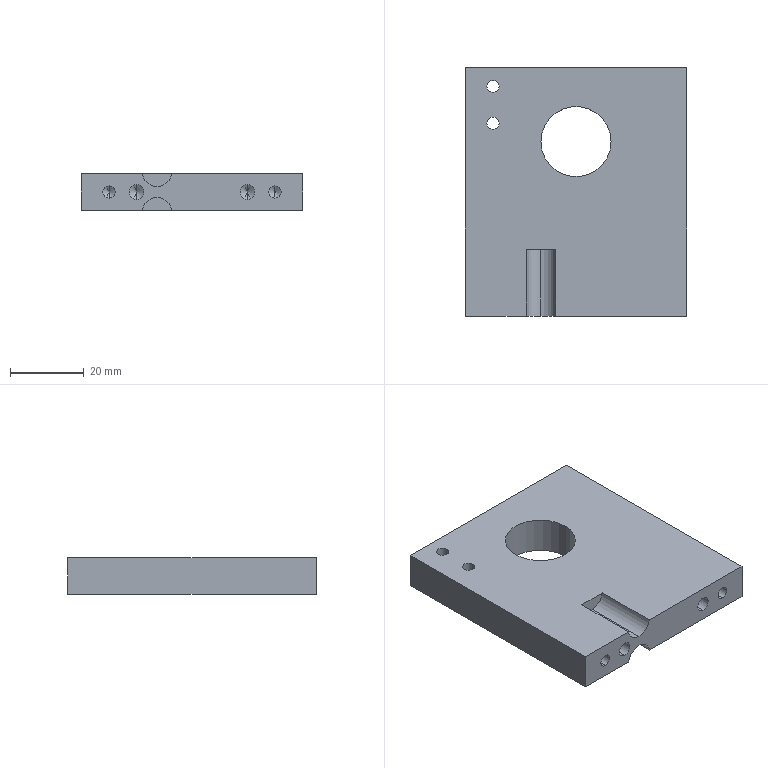Part | STEP file | 11-FG-B03511 | 1 solid | 53 faces | box 60 x 67.3 x 10 mm | volume 35980 mm3 | cylinder 27 | cone 18 | plane 8 | commonest cylinder face diameters 2.5 x10 3.3 x8 4 x4 8 x3 19 x2
STEP:
#1=CARTESIAN_POINT('',(20.5,44.7,6.5));
#2=VERTEX_POINT('',#1);
#3=CARTESIAN_POINT('',(24.469,44.7,10.));
#4=VERTEX_POINT('',#3);
#5=CARTESIAN_POINT('',(20.5,44.7,10.5));
#6=DIRECTION('',(0.,-1.,0.));
#7=DIRECTION('',(0.,0.,-1.));
#8=AXIS2_PLACEMENT_3D('',#5,#6,#7);
#9=CIRCLE('',#8,4.);
#10=EDGE_CURVE('',#2,#4,#9,.T.);
#11=ORIENTED_EDGE('',*,*,#10,.F.);
#12=CARTESIAN_POINT('',(20.5,26.7,6.5));
#13=VERTEX_POINT('',#12);
#14=CARTESIAN_POINT('',(20.5,44.7,6.5));
#15=DIRECTION('',(0.,-1.,0.));
#16=VECTOR('',#15,1000.);
#17=LINE('',#14,#16);
#18=EDGE_CURVE('',#2,#13,#17,.T.);
#19=ORIENTED_EDGE('',*,*,#18,.T.);
#20=CARTESIAN_POINT('',(24.469,26.7,10.));
#21=VERTEX_POINT('',#20);
#22=CARTESIAN_POINT('',(20.5,26.7,10.5));
#23=DIRECTION('',(0.,1.,0.));
#24=DIRECTION('',(0.,0.,1.));
#25=AXIS2_PLACEMENT_3D('',#22,#23,#24);
#26=CIRCLE('',#25,4.);
#27=EDGE_CURVE('',#21,#13,#26,.T.);
#28=ORIENTED_EDGE('',*,*,#27,.F.);
#29=CARTESIAN_POINT('',(24.469,44.7,10.));
#30=DIRECTION('',(0.,-1.,0.));
#31=VECTOR('',#30,1000.);
#32=LINE('',#29,#31);
#33=EDGE_CURVE('',#4,#21,#32,.T.);
#34=ORIENTED_EDGE('',*,*,#33,.F.);
#35=EDGE_LOOP('',(#11,#19,#28,#34));
#36=FACE_OUTER_BOUND('',#35,.T.);
#37=CARTESIAN_POINT('',(20.5,44.7,10.5));
#38=DIRECTION('',(0.,-1.,0.));
#39=DIRECTION('',(0.,0.,-1.));
#40=AXIS2_PLACEMENT_3D('',#37,#38,#39);
#41=CYLINDRICAL_SURFACE('',#40,4.);
#42=ADVANCED_FACE('',(#36),#41,.F.);
#43=CARTESIAN_POINT('',(45.,36.8,7.));
#44=VERTEX_POINT('',#43);
#45=CARTESIAN_POINT('',(45.,36.8,3.));
#46=VERTEX_POINT('',#45);
#47=CARTESIAN_POINT('',(45.,36.8,5.));
#48=DIRECTION('',(0.,-1.,0.));
#49=DIRECTION('',(0.,0.,-1.));
#50=AXIS2_PLACEMENT_3D('',#47,#48,#49);
#51=CIRCLE('',#50,2.);
#52=EDGE_CURVE('',#44,#46,#51,.T.);
#53=ORIENTED_EDGE('',*,*,#52,.F.);
#54=CARTESIAN_POINT('',(45.,26.7,7.));
#55=VERTEX_POINT('',#54);
#56=CARTESIAN_POINT('',(45.,26.7,7.));
#57=DIRECTION('',(0.,-1.,0.));
#58=VECTOR('',#57,1000.);
#59=LINE('',#56,#58);
#60=EDGE_CURVE('',#44,#55,#59,.T.);
#61=ORIENTED_EDGE('',*,*,#60,.T.);
#62=CARTESIAN_POINT('',(45.,26.7,3.));
#63=VERTEX_POINT('',#62);
#64=CARTESIAN_POINT('',(45.,26.7,5.));
#65=DIRECTION('',(0.,-1.,0.));
#66=DIRECTION('',(0.,0.,-1.));
#67=AXIS2_PLACEMENT_3D('',#64,#65,#66);
#68=CIRCLE('',#67,2.);
#69=EDGE_CURVE('',#55,#63,#68,.T.);
#70=ORIENTED_EDGE('',*,*,#69,.T.);
#71=CARTESIAN_POINT('',(45.,26.7,3.));
#72=DIRECTION('',(0.,-1.,0.));
#73=VECTOR('',#72,1000.);
#74=LINE('',#71,#73);
#75=EDGE_CURVE('',#46,#63,#74,.T.);
#76=ORIENTED_EDGE('',*,*,#75,.F.);
#77=EDGE_LOOP('',(#53,#61,#70,#76));
#78=FACE_OUTER_BOUND('',#77,.T.);
#79=CARTESIAN_POINT('',(45.,26.7,5.));
#80=DIRECTION('',(0.,-1.,0.));
#81=DIRECTION('',(0.,0.,-1.));
#82=AXIS2_PLACEMENT_3D('',#79,#80,#81);
#83=CYLINDRICAL_SURFACE('',#82,2.);
#84=ADVANCED_FACE('',(#78),#83,.F.);
#85=CARTESIAN_POINT('',(45.,38.002,5.));
#86=VERTEX_POINT('',#85);
#87=CARTESIAN_POINT('',(45.,36.8,3.));
#88=DIRECTION('',(0.,-0.515,-0.8572));
#89=VECTOR('',#88,1000.);
#90=LINE('',#87,#89);
#91=EDGE_CURVE('',#86,#46,#90,.T.);
#92=ORIENTED_EDGE('',*,*,#91,.F.);
#93=CARTESIAN_POINT('',(45.,36.8,7.));
#94=DIRECTION('',(0.,-0.515,0.8572));
#95=VECTOR('',#94,1000.);
#96=LINE('',#93,#95);
#97=EDGE_CURVE('',#86,#44,#96,.T.);
#98=ORIENTED_EDGE('',*,*,#97,.T.);
#99=ORIENTED_EDGE('',*,*,#52,.T.);
#100=EDGE_LOOP('',(#92,#98,#99));
#101=FACE_OUTER_BOUND('',#100,.T.);
#102=CARTESIAN_POINT('',(45.,36.8,5.));
#103=DIRECTION('',(0.,-1.,0.));
#104=DIRECTION('',(0.,0.,-1.));
#105=AXIS2_PLACEMENT_3D('',#102,#103,#104);
#106=CONICAL_SURFACE('',#105,2.,1.03);
#107=ADVANCED_FACE('',(#101),#106,.F.);
#108=CARTESIAN_POINT('',(15.,36.8,7.));
#109=VERTEX_POINT('',#108);
#110=CARTESIAN_POINT('',(15.,36.8,3.));
#111=VERTEX_POINT('',#110);
#112=CARTESIAN_POINT('',(15.,36.8,5.));
#113=DIRECTION('',(0.,-1.,0.));
#114=DIRECTION('',(0.,0.,-1.));
#115=AXIS2_PLACEMENT_3D('',#112,#113,#114);
#116=CIRCLE('',#115,2.);
#117=EDGE_CURVE('',#109,#111,#116,.T.);
#118=ORIENTED_EDGE('',*,*,#117,.F.);
#119=CARTESIAN_POINT('',(15.,26.7,7.));
#120=VERTEX_POINT('',#119);
#121=CARTESIAN_POINT('',(15.,26.7,7.));
#122=DIRECTION('',(0.,-1.,0.));
#123=VECTOR('',#122,1000.);
#124=LINE('',#121,#123);
#125=EDGE_CURVE('',#109,#120,#124,.T.);
#126=ORIENTED_EDGE('',*,*,#125,.T.);
#127=CARTESIAN_POINT('',(15.,26.7,3.));
#128=VERTEX_POINT('',#127);
#129=CARTESIAN_POINT('',(15.,26.7,5.));
#130=DIRECTION('',(0.,-1.,0.));
#131=DIRECTION('',(0.,0.,-1.));
#132=AXIS2_PLACEMENT_3D('',#129,#130,#131);
#133=CIRCLE('',#132,2.);
#134=EDGE_CURVE('',#120,#128,#133,.T.);
#135=ORIENTED_EDGE('',*,*,#134,.T.);
#136=CARTESIAN_POINT('',(15.,26.7,3.));
#137=DIRECTION('',(0.,-1.,0.));
#138=VECTOR('',#137,1000.);
#139=LINE('',#136,#138);
#140=EDGE_CURVE('',#111,#128,#139,.T.);
#141=ORIENTED_EDGE('',*,*,#140,.F.);
#142=EDGE_LOOP('',(#118,#126,#135,#141));
#143=FACE_OUTER_BOUND('',#142,.T.);
#144=CARTESIAN_POINT('',(15.,26.7,5.));
#145=DIRECTION('',(0.,-1.,0.));
#146=DIRECTION('',(0.,0.,-1.));
#147=AXIS2_PLACEMENT_3D('',#144,#145,#146);
#148=CYLINDRICAL_SURFACE('',#147,2.);
#149=ADVANCED_FACE('',(#143),#148,.F.);
#150=CARTESIAN_POINT('',(15.,38.002,5.));
#151=VERTEX_POINT('',#150);
#152=CARTESIAN_POINT('',(15.,36.8,3.));
#153=DIRECTION('',(0.,-0.515,-0.8572));
#154=VECTOR('',#153,1000.);
#155=LINE('',#152,#154);
#156=EDGE_CURVE('',#151,#111,#155,.T.);
#157=ORIENTED_EDGE('',*,*,#156,.F.);
#158=CARTESIAN_POINT('',(15.,36.8,7.));
#159=DIRECTION('',(0.,-0.515,0.8572));
#160=VECTOR('',#159,1000.);
#161=LINE('',#158,#160);
#162=EDGE_CURVE('',#151,#109,#161,.T.);
#163=ORIENTED_EDGE('',*,*,#162,.T.);
#164=ORIENTED_EDGE('',*,*,#117,.T.);
#165=EDGE_LOOP('',(#157,#163,#164));
#166=FACE_OUTER_BOUND('',#165,.T.);
#167=CARTESIAN_POINT('',(15.,36.8,5.));
#168=DIRECTION('',(0.,-1.,0.));
#169=DIRECTION('',(0.,0.,-1.));
#170=AXIS2_PLACEMENT_3D('',#167,#168,#169);
#171=CONICAL_SURFACE('',#170,2.,1.03);
#172=ADVANCED_FACE('',(#166),#171,.F.);
#173=CARTESIAN_POINT('',(52.5,36.8,6.65));
#174=VERTEX_POINT('',#173);
#175=CARTESIAN_POINT('',(52.5,36.8,3.35));
#176=VERTEX_POINT('',#175);
#177=CARTESIAN_POINT('',(52.5,36.8,5.));
#178=DIRECTION('',(0.,-1.,0.));
#179=DIRECTION('',(0.,0.,-1.));
#180=AXIS2_PLACEMENT_3D('',#177,#178,#179);
#181=CIRCLE('',#180,1.65);
#182=EDGE_CURVE('',#174,#176,#181,.T.);
#183=ORIENTED_EDGE('',*,*,#182,.F.);
#184=CARTESIAN_POINT('',(52.5,26.7,6.65));
#185=VERTEX_POINT('',#184);
#186=CARTESIAN_POINT('',(52.5,26.7,6.65));
#187=DIRECTION('',(0.,-1.,0.));
#188=VECTOR('',#187,1000.);
#189=LINE('',#186,#188);
#190=EDGE_CURVE('',#174,#185,#189,.T.);
#191=ORIENTED_EDGE('',*,*,#190,.T.);
#192=CARTESIAN_POINT('',(52.5,26.7,3.35));
#193=VERTEX_POINT('',#192);
#194=CARTESIAN_POINT('',(52.5,26.7,5.));
#195=DIRECTION('',(0.,-1.,0.));
#196=DIRECTION('',(0.,0.,-1.));
#197=AXIS2_PLACEMENT_3D('',#194,#195,#196);
#198=CIRCLE('',#197,1.65);
#199=EDGE_CURVE('',#185,#193,#198,.T.);
#200=ORIENTED_EDGE('',*,*,#199,.T.);
#201=CARTESIAN_POINT('',(52.5,26.7,3.35));
#202=DIRECTION('',(0.,-1.,0.));
#203=VECTOR('',#202,1000.);
#204=LINE('',#201,#203);
#205=EDGE_CURVE('',#176,#193,#204,.T.);
#206=ORIENTED_EDGE('',*,*,#205,.F.);
#207=EDGE_LOOP('',(#183,#191,#200,#206));
#208=FACE_OUTER_BOUND('',#207,.T.);
#209=CARTESIAN_POINT('',(52.5,26.7,5.));
#210=DIRECTION('',(0.,-1.,0.));
#211=DIRECTION('',(0.,0.,-1.));
#212=AXIS2_PLACEMENT_3D('',#209,#210,#211);
#213=CYLINDRICAL_SURFACE('',#212,1.65);
#214=ADVANCED_FACE('',(#208),#213,.F.);
#215=CARTESIAN_POINT('',(52.5,37.752,5.066));
#216=VERTEX_POINT('',#215);
#217=CARTESIAN_POINT('',(52.5,37.752,4.934));
#218=VERTEX_POINT('',#217);
#219=CARTESIAN_POINT('',(52.5,37.752,5.066));
#220=CARTESIAN_POINT('',(52.496,37.759,5.055));
#221=CARTESIAN_POINT('',(52.491,37.765,5.043));
#222=CARTESIAN_POINT('',(52.487,37.771,5.031));
#223=CARTESIAN_POINT('',(52.486,37.774,5.025));
#224=CARTESIAN_POINT('',(52.484,37.776,5.02));
#225=CARTESIAN_POINT('',(52.483,37.778,5.014));
#226=CARTESIAN_POINT('',(52.482,37.78,5.01));
#227=CARTESIAN_POINT('',(52.482,37.78,5.005));
#228=CARTESIAN_POINT('',(52.482,37.78,5.001));
#229=CARTESIAN_POINT('',(52.482,37.78,4.996));
#230=CARTESIAN_POINT('',(52.482,37.78,4.991));
#231=CARTESIAN_POINT('',(52.483,37.779,4.987));
#232=CARTESIAN_POINT('',(52.486,37.774,4.972));
#233=CARTESIAN_POINT('',(52.491,37.766,4.958));
#234=CARTESIAN_POINT('',(52.496,37.758,4.945));
#235=CARTESIAN_POINT('',(52.497,37.756,4.941));
#236=CARTESIAN_POINT('',(52.499,37.754,4.938));
#237=CARTESIAN_POINT('',(52.5,37.752,4.934));
#238=B_SPLINE_CURVE_WITH_KNOTS('',3,(#219,#220,#221,#222,#223,#224,#225,#226,#227,#228,#229,#230,#231,#232,#233,#234,#235,#236,#237),.UNSPECIFIED.,.F.,.F.,(4,3,3,3,3,3,4),(0.000000627,0.00004275,0.0000616,0.00007533,0.00008914,0.0001384,0.0001519),.UNSPECIFIED.);
#239=EDGE_CURVE('',#216,#218,#238,.T.);
#240=ORIENTED_EDGE('',*,*,#239,.F.);
#241=CARTESIAN_POINT('',(52.5,36.8,6.65));
#242=DIRECTION('',(0.,-0.515,0.8572));
#243=VECTOR('',#242,1000.);
#244=LINE('',#241,#243);
#245=EDGE_CURVE('',#216,#174,#244,.T.);
#246=ORIENTED_EDGE('',*,*,#245,.T.);
#247=ORIENTED_EDGE('',*,*,#182,.T.);
#248=CARTESIAN_POINT('',(52.5,36.8,3.35));
#249=DIRECTION('',(0.,-0.515,-0.8572));
#250=VECTOR('',#249,1000.);
#251=LINE('',#248,#250);
#252=EDGE_CURVE('',#218,#176,#251,.T.);
#253=ORIENTED_EDGE('',*,*,#252,.F.);
#254=EDGE_LOOP('',(#240,#246,#247,#253));
#255=FACE_OUTER_BOUND('',#254,.T.);
#256=CARTESIAN_POINT('',(52.5,36.8,5.));
#257=DIRECTION('',(0.,-1.,0.));
#258=DIRECTION('',(0.,0.,-1.));
#259=AXIS2_PLACEMENT_3D('',#256,#257,#258);
#260=CONICAL_SURFACE('',#259,1.65,1.03);
#261=ADVANCED_FACE('',(#255),#260,.F.);
#262=CARTESIAN_POINT('',(7.5,36.8,6.65));
#263=VERTEX_POINT('',#262);
#264=CARTESIAN_POINT('',(7.5,36.8,3.35));
#265=VERTEX_POINT('',#264);
#266=CARTESIAN_POINT('',(7.5,36.8,5.));
#267=DIRECTION('',(0.,-1.,0.));
#268=DIRECTION('',(0.,0.,-1.));
#269=AXIS2_PLACEMENT_3D('',#266,#267,#268);
#270=CIRCLE('',#269,1.65);
#271=EDGE_CURVE('',#263,#265,#270,.T.);
#272=ORIENTED_EDGE('',*,*,#271,.F.);
#273=CARTESIAN_POINT('',(7.5,26.7,6.65));
#274=VERTEX_POINT('',#273);
#275=CARTESIAN_POINT('',(7.5,26.7,6.65));
#276=DIRECTION('',(0.,-1.,0.));
#277=VECTOR('',#276,1000.);
#278=LINE('',#275,#277);
#279=EDGE_CURVE('',#263,#274,#278,.T.);
#280=ORIENTED_EDGE('',*,*,#279,.T.);
#281=CARTESIAN_POINT('',(7.5,26.7,3.35));
#282=VERTEX_POINT('',#281);
#283=CARTESIAN_POINT('',(7.5,26.7,5.));
#284=DIRECTION('',(0.,-1.,0.));
#285=DIRECTION('',(0.,0.,-1.));
#286=AXIS2_PLACEMENT_3D('',#283,#284,#285);
#287=CIRCLE('',#286,1.65);
#288=EDGE_CURVE('',#274,#282,#287,.T.);
#289=ORIENTED_EDGE('',*,*,#288,.T.);
#290=CARTESIAN_POINT('',(7.5,26.7,3.35));
#291=DIRECTION('',(0.,-1.,0.));
#292=VECTOR('',#291,1000.);
#293=LINE('',#290,#292);
#294=EDGE_CURVE('',#265,#282,#293,.T.);
#295=ORIENTED_EDGE('',*,*,#294,.F.);
#296=EDGE_LOOP('',(#272,#280,#289,#295));
#297=FACE_OUTER_BOUND('',#296,.T.);
#298=CARTESIAN_POINT('',(7.5,26.7,5.));
#299=DIRECTION('',(0.,-1.,0.));
#300=DIRECTION('',(0.,0.,-1.));
#301=AXIS2_PLACEMENT_3D('',#298,#299,#300);
#302=CYLINDRICAL_SURFACE('',#301,1.65);
#303=ADVANCED_FACE('',(#297),#302,.F.);
#304=CARTESIAN_POINT('',(7.5,37.791,5.));
#305=VERTEX_POINT('',#304);
#306=CARTESIAN_POINT('',(7.5,36.8,3.35));
#307=DIRECTION('',(0.,-0.515,-0.8572));
#308=VECTOR('',#307,1000.);
#309=LINE('',#306,#308);
#310=EDGE_CURVE('',#305,#265,#309,.T.);
#311=ORIENTED_EDGE('',*,*,#310,.F.);
#312=CARTESIAN_POINT('',(7.5,36.8,6.65));
#313=DIRECTION('',(0.,-0.515,0.8572));
#314=VECTOR('',#313,1000.);
#315=LINE('',#312,#314);
#316=EDGE_CURVE('',#305,#263,#315,.T.);
#317=ORIENTED_EDGE('',*,*,#316,.T.);
#318=ORIENTED_EDGE('',*,*,#271,.T.);
#319=EDGE_LOOP('',(#311,#317,#318));
#320=FACE_OUTER_BOUND('',#319,.T.);
#321=CARTESIAN_POINT('',(7.5,36.8,5.));
#322=DIRECTION('',(0.,-1.,0.));
#323=DIRECTION('',(0.,0.,-1.));
#324=AXIS2_PLACEMENT_3D('',#321,#322,#323);
#325=CONICAL_SURFACE('',#324,1.65,1.03);
#326=ADVANCED_FACE('',(#320),#325,.F.);
#327=CARTESIAN_POINT('',(52.5,39.,6.25));
#328=VERTEX_POINT('',#327);
#329=CARTESIAN_POINT('',(52.5,39.,5.));
#330=DIRECTION('',(1.,0.,0.));
#331=DIRECTION('',(0.,0.,-1.));
#332=AXIS2_PLACEMENT_3D('',#329,#330,#331);
#333=CIRCLE('',#332,1.25);
#334=EDGE_CURVE('',#328,#216,#333,.T.);
#335=ORIENTED_EDGE('',*,*,#334,.F.);
#336=CARTESIAN_POINT('',(60.,39.,6.25));
#337=VERTEX_POINT('',#336);
#338=CARTESIAN_POINT('',(60.,39.,6.25));
#339=DIRECTION('',(1.,0.,0.));
#340=VECTOR('',#339,1000.);
#341=LINE('',#338,#340);
#342=EDGE_CURVE('',#328,#337,#341,.T.);
#343=ORIENTED_EDGE('',*,*,#342,.T.);
#344=CARTESIAN_POINT('',(60.,39.,3.75));
#345=VERTEX_POINT('',#344);
#346=CARTESIAN_POINT('',(60.,39.,5.));
#347=DIRECTION('',(1.,0.,0.));
#348=DIRECTION('',(0.,0.,-1.));
#349=AXIS2_PLACEMENT_3D('',#346,#347,#348);
#350=CIRCLE('',#349,1.25);
#351=EDGE_CURVE('',#337,#345,#350,.T.);
#352=ORIENTED_EDGE('',*,*,#351,.T.);
#353=CARTESIAN_POINT('',(52.5,39.,3.75));
#354=VERTEX_POINT('',#353);
#355=CARTESIAN_POINT('',(60.,39.,3.75));
#356=DIRECTION('',(1.,0.,0.));
#357=VECTOR('',#356,1000.);
#358=LINE('',#355,#357);
#359=EDGE_CURVE('',#354,#345,#358,.T.);
#360=ORIENTED_EDGE('',*,*,#359,.F.);
#361=CARTESIAN_POINT('',(52.5,39.,5.));
#362=DIRECTION('',(1.,0.,0.));
#363=DIRECTION('',(0.,0.,-1.));
#364=AXIS2_PLACEMENT_3D('',#361,#362,#363);
#365=CIRCLE('',#364,1.25);
#366=EDGE_CURVE('',#218,#354,#365,.T.);
#367=ORIENTED_EDGE('',*,*,#366,.F.);
#368=CARTESIAN_POINT('',(52.5,37.752,4.934));
#369=CARTESIAN_POINT('',(52.505,37.752,4.934));
#370=CARTESIAN_POINT('',(52.509,37.752,4.934));
#371=CARTESIAN_POINT('',(52.514,37.752,4.935));
#372=CARTESIAN_POINT('',(52.522,37.752,4.937));
#373=CARTESIAN_POINT('',(52.529,37.751,4.94));
#374=CARTESIAN_POINT('',(52.536,37.751,4.944));
#375=CARTESIAN_POINT('',(52.543,37.751,4.948));
#376=CARTESIAN_POINT('',(52.549,37.751,4.953));
#377=CARTESIAN_POINT('',(52.554,37.751,4.959));
#378=CARTESIAN_POINT('',(52.559,37.75,4.965));
#379=CARTESIAN_POINT('',(52.563,37.75,4.972));
#380=CARTESIAN_POINT('',(52.565,37.75,4.979));
#381=CARTESIAN_POINT('',(52.568,37.75,4.986));
#382=CARTESIAN_POINT('',(52.569,37.75,4.994));
#383=CARTESIAN_POINT('',(52.569,37.75,5.001));
#384=CARTESIAN_POINT('',(52.569,37.75,5.008));
#385=CARTESIAN_POINT('',(52.567,37.75,5.015));
#386=CARTESIAN_POINT('',(52.565,37.75,5.022));
#387=CARTESIAN_POINT('',(52.563,37.75,5.029));
#388=CARTESIAN_POINT('',(52.559,37.75,5.035));
#389=CARTESIAN_POINT('',(52.554,37.751,5.04));
#390=CARTESIAN_POINT('',(52.55,37.751,5.046));
#391=CARTESIAN_POINT('',(52.544,37.751,5.051));
#392=CARTESIAN_POINT('',(52.538,37.751,5.055));
#393=CARTESIAN_POINT('',(52.532,37.751,5.059));
#394=CARTESIAN_POINT('',(52.525,37.752,5.062));
#395=CARTESIAN_POINT('',(52.517,37.752,5.064));
#396=CARTESIAN_POINT('',(52.512,37.752,5.065));
#397=CARTESIAN_POINT('',(52.506,37.752,5.066));
#398=CARTESIAN_POINT('',(52.5,37.752,5.066));
#399=B_SPLINE_CURVE_WITH_KNOTS('',3,(#368,#369,#370,#371,#372,#373,#374,#375,#376,#377,#378,#379,#380,#381,#382,#383,#384,#385,#386,#387,#388,#389,#390,#391,#392,#393,#394,#395,#396,#397,#398),.UNSPECIFIED.,.F.,.F.,(4,3,3,3,3,3,3,3,3,3,4),(0.00005605,0.00006989,0.00009398,0.0001177,0.0001407,0.0001626,0.0001839,0.0002051,0.000227,0.0002498,0.0002671),.UNSPECIFIED.);
#400=EDGE_CURVE('',#218,#216,#399,.T.);
#401=ORIENTED_EDGE('',*,*,#400,.T.);
#402=EDGE_LOOP('',(#335,#343,#352,#360,#367,#401));
#403=FACE_OUTER_BOUND('',#402,.T.);
#404=CARTESIAN_POINT('',(60.,39.,5.));
#405=DIRECTION('',(1.,0.,0.));
#406=DIRECTION('',(0.,0.,-1.));
#407=AXIS2_PLACEMENT_3D('',#404,#405,#406);
#408=CYLINDRICAL_SURFACE('',#407,1.25);
#409=ADVANCED_FACE('',(#403),#408,.F.);
#410=CARTESIAN_POINT('',(51.749,39.,5.));
#411=VERTEX_POINT('',#410);
#412=CARTESIAN_POINT('',(52.5,39.,3.75));
#413=DIRECTION('',(0.515,0.,-0.8572));
#414=VECTOR('',#413,1000.);
#415=LINE('',#412,#414);
#416=EDGE_CURVE('',#411,#354,#415,.T.);
#417=ORIENTED_EDGE('',*,*,#416,.F.);
#418=CARTESIAN_POINT('',(52.5,39.,6.25));
#419=DIRECTION('',(0.515,0.,0.8572));
#420=VECTOR('',#419,1000.);
#421=LINE('',#418,#420);
#422=EDGE_CURVE('',#411,#328,#421,.T.);
#423=ORIENTED_EDGE('',*,*,#422,.T.);
#424=ORIENTED_EDGE('',*,*,#334,.T.);
#425=ORIENTED_EDGE('',*,*,#239,.T.);
#426=ORIENTED_EDGE('',*,*,#366,.T.);
#427=EDGE_LOOP('',(#417,#423,#424,#425,#426));
#428=FACE_OUTER_BOUND('',#427,.T.);
#429=CARTESIAN_POINT('',(52.5,39.,5.));
#430=DIRECTION('',(1.,0.,0.));
#431=DIRECTION('',(0.,0.,-1.));
#432=AXIS2_PLACEMENT_3D('',#429,#430,#431);
#433=CONICAL_SURFACE('',#432,1.25,1.03);
#434=ADVANCED_FACE('',(#428),#433,.F.);
#435=CARTESIAN_POINT('',(52.5,49.,6.25));
#436=VERTEX_POINT('',#435);
#437=CARTESIAN_POINT('',(52.5,49.,3.75));
#438=VERTEX_POINT('',#437);
#439=CARTESIAN_POINT('',(52.5,49.,5.));
#440=DIRECTION('',(1.,0.,0.));
#441=DIRECTION('',(0.,0.,-1.));
#442=AXIS2_PLACEMENT_3D('',#439,#440,#441);
#443=CIRCLE('',#442,1.25);
#444=EDGE_CURVE('',#436,#438,#443,.T.);
#445=ORIENTED_EDGE('',*,*,#444,.F.);
#446=CARTESIAN_POINT('',(60.,49.,6.25));
#447=VERTEX_POINT('',#446);
#448=CARTESIAN_POINT('',(60.,49.,6.25));
#449=DIRECTION('',(1.,0.,0.));
#450=VECTOR('',#449,1000.);
#451=LINE('',#448,#450);
#452=EDGE_CURVE('',#436,#447,#451,.T.);
#453=ORIENTED_EDGE('',*,*,#452,.T.);
#454=CARTESIAN_POINT('',(60.,49.,3.75));
#455=VERTEX_POINT('',#454);
#456=CARTESIAN_POINT('',(60.,49.,5.));
#457=DIRECTION('',(1.,0.,0.));
#458=DIRECTION('',(0.,0.,-1.));
#459=AXIS2_PLACEMENT_3D('',#456,#457,#458);
#460=CIRCLE('',#459,1.25);
#461=EDGE_CURVE('',#447,#455,#460,.T.);
#462=ORIENTED_EDGE('',*,*,#461,.T.);
#463=CARTESIAN_POINT('',(60.,49.,3.75));
#464=DIRECTION('',(1.,0.,0.));
#465=VECTOR('',#464,1000.);
#466=LINE('',#463,#465);
#467=EDGE_CURVE('',#438,#455,#466,.T.);
#468=ORIENTED_EDGE('',*,*,#467,.F.);
#469=EDGE_LOOP('',(#445,#453,#462,#468));
#470=FACE_OUTER_BOUND('',#469,.T.);
#471=CARTESIAN_POINT('',(60.,49.,5.));
#472=DIRECTION('',(1.,0.,0.));
#473=DIRECTION('',(0.,0.,-1.));
#474=AXIS2_PLACEMENT_3D('',#471,#472,#473);
#475=CYLINDRICAL_SURFACE('',#474,1.25);
#476=ADVANCED_FACE('',(#470),#475,.F.);
#477=CARTESIAN_POINT('',(51.749,49.,5.));
#478=VERTEX_POINT('',#477);
#479=CARTESIAN_POINT('',(52.5,49.,3.75));
#480=DIRECTION('',(0.515,0.,-0.8572));
#481=VECTOR('',#480,1000.);
#482=LINE('',#479,#481);
#483=EDGE_CURVE('',#478,#438,#482,.T.);
#484=ORIENTED_EDGE('',*,*,#483,.F.);
#485=CARTESIAN_POINT('',(52.5,49.,6.25));
#486=DIRECTION('',(0.515,0.,0.8572));
#487=VECTOR('',#486,1000.);
#488=LINE('',#485,#487);
#489=EDGE_CURVE('',#478,#436,#488,.T.);
#490=ORIENTED_EDGE('',*,*,#489,.T.);
#491=ORIENTED_EDGE('',*,*,#444,.T.);
#492=EDGE_LOOP('',(#484,#490,#491));
#493=FACE_OUTER_BOUND('',#492,.T.);
#494=CARTESIAN_POINT('',(52.5,49.,5.));
#495=DIRECTION('',(1.,0.,0.));
#496=DIRECTION('',(0.,0.,-1.));
#497=AXIS2_PLACEMENT_3D('',#494,#495,#496);
#498=CONICAL_SURFACE('',#497,1.25,1.03);
#499=ADVANCED_FACE('',(#493),#498,.F.);
#500=CARTESIAN_POINT('',(52.5,59.,6.25));
#501=VERTEX_POINT('',#500);
#502=CARTESIAN_POINT('',(52.5,59.,3.75));
#503=VERTEX_POINT('',#502);
#504=CARTESIAN_POINT('',(52.5,59.,5.));
#505=DIRECTION('',(1.,0.,0.));
#506=DIRECTION('',(0.,0.,-1.));
#507=AXIS2_PLACEMENT_3D('',#504,#505,#506);
#508=CIRCLE('',#507,1.25);
#509=EDGE_CURVE('',#501,#503,#508,.T.);
#510=ORIENTED_EDGE('',*,*,#509,.F.);
#511=CARTESIAN_POINT('',(60.,59.,6.25));
#512=VERTEX_POINT('',#511);
#513=CARTESIAN_POINT('',(60.,59.,6.25));
#514=DIRECTION('',(1.,0.,0.));
#515=VECTOR('',#514,1000.);
#516=LINE('',#513,#515);
#517=EDGE_CURVE('',#501,#512,#516,.T.);
#518=ORIENTED_EDGE('',*,*,#517,.T.);
#519=CARTESIAN_POINT('',(60.,59.,3.75));
#520=VERTEX_POINT('',#519);
#521=CARTESIAN_POINT('',(60.,59.,5.));
#522=DIRECTION('',(1.,0.,0.));
#523=DIRECTION('',(0.,0.,-1.));
#524=AXIS2_PLACEMENT_3D('',#521,#522,#523);
#525=CIRCLE('',#524,1.25);
#526=EDGE_CURVE('',#512,#520,#525,.T.);
#527=ORIENTED_EDGE('',*,*,#526,.T.);
#528=CARTESIAN_POINT('',(60.,59.,3.75));
#529=DIRECTION('',(1.,0.,0.));
#530=VECTOR('',#529,1000.);
#531=LINE('',#528,#530);
#532=EDGE_CURVE('',#503,#520,#531,.T.);
#533=ORIENTED_EDGE('',*,*,#532,.F.);
#534=EDGE_LOOP('',(#510,#518,#527,#533));
#535=FACE_OUTER_BOUND('',#534,.T.);
#536=CARTESIAN_POINT('',(60.,59.,5.));
#537=DIRECTION('',(1.,0.,0.));
#538=DIRECTION('',(0.,0.,-1.));
#539=AXIS2_PLACEMENT_3D('',#536,#537,#538);
#540=CYLINDRICAL_SURFACE('',#539,1.25);
#541=ADVANCED_FACE('',(#535),#540,.F.);
#542=CARTESIAN_POINT('',(51.749,59.,5.));
#543=VERTEX_POINT('',#542);
#544=CARTESIAN_POINT('',(52.5,59.,3.75));
#545=DIRECTION('',(0.515,0.,-0.8572));
#546=VECTOR('',#545,1000.);
#547=LINE('',#544,#546);
#548=EDGE_CURVE('',#543,#503,#547,.T.);
#549=ORIENTED_EDGE('',*,*,#548,.F.);
#550=CARTESIAN_POINT('',(52.5,59.,6.25));
#551=DIRECTION('',(0.515,0.,0.8572));
#552=VECTOR('',#551,1000.);
#553=LINE('',#550,#552);
#554=EDGE_CURVE('',#543,#501,#553,.T.);
#555=ORIENTED_EDGE('',*,*,#554,.T.);
#556=ORIENTED_EDGE('',*,*,#509,.T.);
#557=EDGE_LOOP('',(#549,#555,#556));
#558=FACE_OUTER_BOUND('',#557,.T.);
#559=CARTESIAN_POINT('',(52.5,59.,5.));
#560=DIRECTION('',(1.,0.,0.));
#561=DIRECTION('',(0.,0.,-1.));
#562=AXIS2_PLACEMENT_3D('',#559,#560,#561);
#563=CONICAL_SURFACE('',#562,1.25,1.03);
#564=ADVANCED_FACE('',(#558),#563,.F.);
#565=CARTESIAN_POINT('',(52.5,69.,6.25));
#566=VERTEX_POINT('',#565);
#567=CARTESIAN_POINT('',(52.5,69.,3.75));
#568=VERTEX_POINT('',#567);
#569=CARTESIAN_POINT('',(52.5,69.,5.));
#570=DIRECTION('',(1.,0.,0.));
#571=DIRECTION('',(0.,0.,-1.));
#572=AXIS2_PLACEMENT_3D('',#569,#570,#571);
#573=CIRCLE('',#572,1.25);
#574=EDGE_CURVE('',#566,#568,#573,.T.);
#575=ORIENTED_EDGE('',*,*,#574,.F.);
#576=CARTESIAN_POINT('',(60.,69.,6.25));
#577=VERTEX_POINT('',#576);
#578=CARTESIAN_POINT('',(60.,69.,6.25));
#579=DIRECTION('',(1.,0.,0.));
#580=VECTOR('',#579,1000.);
#581=LINE('',#578,#580);
#582=EDGE_CURVE('',#566,#577,#581,.T.);
#583=ORIENTED_EDGE('',*,*,#582,.T.);
#584=CARTESIAN_POINT('',(60.,69.,3.75));
#585=VERTEX_POINT('',#584);
#586=CARTESIAN_POINT('',(60.,69.,5.));
#587=DIRECTION('',(1.,0.,0.));
#588=DIRECTION('',(0.,0.,-1.));
#589=AXIS2_PLACEMENT_3D('',#586,#587,#588);
#590=CIRCLE('',#589,1.25);
#591=EDGE_CURVE('',#577,#585,#590,.T.);
#592=ORIENTED_EDGE('',*,*,#591,.T.);
#593=CARTESIAN_POINT('',(60.,69.,3.75));
#594=DIRECTION('',(1.,0.,0.));
#595=VECTOR('',#594,1000.);
#596=LINE('',#593,#595);
#597=EDGE_CURVE('',#568,#585,#596,.T.);
#598=ORIENTED_EDGE('',*,*,#597,.F.);
#599=EDGE_LOOP('',(#575,#583,#592,#598));
#600=FACE_OUTER_BOUND('',#599,.T.);
#601=CARTESIAN_POINT('',(60.,69.,5.));
#602=DIRECTION('',(1.,0.,0.));
#603=DIRECTION('',(0.,0.,-1.));
#604=AXIS2_PLACEMENT_3D('',#601,#602,#603);
#605=CYLINDRICAL_SURFACE('',#604,1.25);
#606=ADVANCED_FACE('',(#600),#605,.F.);
#607=CARTESIAN_POINT('',(51.749,69.,5.));
#608=VERTEX_POINT('',#607);
#609=CARTESIAN_POINT('',(52.5,69.,3.75));
#610=DIRECTION('',(0.515,0.,-0.8572));
#611=VECTOR('',#610,1000.);
#612=LINE('',#609,#611);
#613=EDGE_CURVE('',#608,#568,#612,.T.);
#614=ORIENTED_EDGE('',*,*,#613,.F.);
#615=CARTESIAN_POINT('',(52.5,69.,6.25));
#616=DIRECTION('',(0.515,0.,0.8572));
#617=VECTOR('',#616,1000.);
#618=LINE('',#615,#617);
#619=EDGE_CURVE('',#608,#566,#618,.T.);
#620=ORIENTED_EDGE('',*,*,#619,.T.);
#621=ORIENTED_EDGE('',*,*,#574,.T.);
#622=EDGE_LOOP('',(#614,#620,#621));
#623=FACE_OUTER_BOUND('',#622,.T.);
#624=CARTESIAN_POINT('',(52.5,69.,5.));
#625=DIRECTION('',(1.,0.,0.));
#626=DIRECTION('',(0.,0.,-1.));
#627=AXIS2_PLACEMENT_3D('',#624,#625,#626);
#628=CONICAL_SURFACE('',#627,1.25,1.03);
#629=ADVANCED_FACE('',(#623),#628,.F.);
#630=CARTESIAN_POINT('',(52.5,79.,6.25));
#631=VERTEX_POINT('',#630);
#632=CARTESIAN_POINT('',(52.5,79.,3.75));
#633=VERTEX_POINT('',#632);
#634=CARTESIAN_POINT('',(52.5,79.,5.));
#635=DIRECTION('',(1.,0.,0.));
#636=DIRECTION('',(0.,0.,-1.));
#637=AXIS2_PLACEMENT_3D('',#634,#635,#636);
#638=CIRCLE('',#637,1.25);
#639=EDGE_CURVE('',#631,#633,#638,.T.);
#640=ORIENTED_EDGE('',*,*,#639,.F.);
#641=CARTESIAN_POINT('',(60.,79.,6.25));
#642=VERTEX_POINT('',#641);
#643=CARTESIAN_POINT('',(60.,79.,6.25));
#644=DIRECTION('',(1.,0.,0.));
#645=VECTOR('',#644,1000.);
#646=LINE('',#643,#645);
#647=EDGE_CURVE('',#631,#642,#646,.T.);
#648=ORIENTED_EDGE('',*,*,#647,.T.);
#649=CARTESIAN_POINT('',(60.,79.,3.75));
#650=VERTEX_POINT('',#649);
#651=CARTESIAN_POINT('',(60.,79.,5.));
#652=DIRECTION('',(1.,0.,0.));
#653=DIRECTION('',(0.,0.,-1.));
#654=AXIS2_PLACEMENT_3D('',#651,#652,#653);
#655=CIRCLE('',#654,1.25);
#656=EDGE_CURVE('',#642,#650,#655,.T.);
#657=ORIENTED_EDGE('',*,*,#656,.T.);
#658=CARTESIAN_POINT('',(60.,79.,3.75));
#659=DIRECTION('',(1.,0.,0.));
#660=VECTOR('',#659,1000.);
#661=LINE('',#658,#660);
#662=EDGE_CURVE('',#633,#650,#661,.T.);
#663=ORIENTED_EDGE('',*,*,#662,.F.);
#664=EDGE_LOOP('',(#640,#648,#657,#663));
#665=FACE_OUTER_BOUND('',#664,.T.);
#666=CARTESIAN_POINT('',(60.,79.,5.));
#667=DIRECTION('',(1.,0.,0.));
#668=DIRECTION('',(0.,0.,-1.));
#669=AXIS2_PLACEMENT_3D('',#666,#667,#668);
#670=CYLINDRICAL_SURFACE('',#669,1.25);
#671=ADVANCED_FACE('',(#665),#670,.F.);
#672=CARTESIAN_POINT('',(51.749,79.,5.));
#673=VERTEX_POINT('',#672);
#674=CARTESIAN_POINT('',(52.5,79.,3.75));
#675=DIRECTION('',(0.515,0.,-0.8572));
#676=VECTOR('',#675,1000.);
#677=LINE('',#674,#676);
#678=EDGE_CURVE('',#673,#633,#677,.T.);
#679=ORIENTED_EDGE('',*,*,#678,.F.);
#680=CARTESIAN_POINT('',(52.5,79.,6.25));
#681=DIRECTION('',(0.515,0.,0.8572));
#682=VECTOR('',#681,1000.);
#683=LINE('',#680,#682);
#684=EDGE_CURVE('',#673,#631,#683,.T.);
#685=ORIENTED_EDGE('',*,*,#684,.T.);
#686=ORIENTED_EDGE('',*,*,#639,.T.);
#687=EDGE_LOOP('',(#679,#685,#686));
#688=FACE_OUTER_BOUND('',#687,.T.);
#689=CARTESIAN_POINT('',(52.5,79.,5.));
#690=DIRECTION('',(1.,0.,0.));
#691=DIRECTION('',(0.,0.,-1.));
#692=AXIS2_PLACEMENT_3D('',#689,#690,#691);
#693=CONICAL_SURFACE('',#692,1.25,1.03);
#694=ADVANCED_FACE('',(#688),#693,.F.);
#695=CARTESIAN_POINT('',(9.15,89.,10.));
#696=VERTEX_POINT('',#695);
#697=CARTESIAN_POINT('',(5.85,89.,10.));
#698=VERTEX_POINT('',#697);
#699=CARTESIAN_POINT('',(7.5,89.,10.));
#700=DIRECTION('',(0.,0.,-1.));
#701=DIRECTION('',(-1.,0.,0.));
#702=AXIS2_PLACEMENT_3D('',#699,#700,#701);
#703=CIRCLE('',#702,1.65);
#704=EDGE_CURVE('',#696,#698,#703,.T.);
#705=ORIENTED_EDGE('',*,*,#704,.F.);
#706=CARTESIAN_POINT('',(9.15,89.,0.));
#707=VERTEX_POINT('',#706);
#708=CARTESIAN_POINT('',(9.15,89.,0.));
#709=DIRECTION('',(0.,0.,-1.));
#710=VECTOR('',#709,1000.);
#711=LINE('',#708,#710);
#712=EDGE_CURVE('',#696,#707,#711,.T.);
#713=ORIENTED_EDGE('',*,*,#712,.T.);
#714=CARTESIAN_POINT('',(5.85,89.,0.));
#715=VERTEX_POINT('',#714);
#716=CARTESIAN_POINT('',(7.5,89.,0.));
#717=DIRECTION('',(0.,0.,-1.));
#718=DIRECTION('',(-1.,0.,0.));
#719=AXIS2_PLACEMENT_3D('',#716,#717,#718);
#720=CIRCLE('',#719,1.65);
#721=EDGE_CURVE('',#707,#715,#720,.T.);
#722=ORIENTED_EDGE('',*,*,#721,.T.);
#723=CARTESIAN_POINT('',(5.85,89.,0.));
#724=DIRECTION('',(0.,0.,-1.));
#725=VECTOR('',#724,1000.);
#726=LINE('',#723,#725);
#727=EDGE_CURVE('',#698,#715,#726,.T.);
#728=ORIENTED_EDGE('',*,*,#727,.F.);
#729=EDGE_LOOP('',(#705,#713,#722,#728));
#730=FACE_OUTER_BOUND('',#729,.T.);
#731=CARTESIAN_POINT('',(7.5,89.,0.));
#732=DIRECTION('',(0.,0.,-1.));
#733=DIRECTION('',(-1.,0.,0.));
#734=AXIS2_PLACEMENT_3D('',#731,#732,#733);
#735=CYLINDRICAL_SURFACE('',#734,1.65);
#736=ADVANCED_FACE('',(#730),#735,.F.);
#737=CARTESIAN_POINT('',(9.15,79.,10.));
#738=VERTEX_POINT('',#737);
#739=CARTESIAN_POINT('',(5.85,79.,10.));
#740=VERTEX_POINT('',#739);
#741=CARTESIAN_POINT('',(7.5,79.,10.));
#742=DIRECTION('',(0.,0.,-1.));
#743=DIRECTION('',(-1.,0.,0.));
#744=AXIS2_PLACEMENT_3D('',#741,#742,#743);
#745=CIRCLE('',#744,1.65);
#746=EDGE_CURVE('',#738,#740,#745,.T.);
#747=ORIENTED_EDGE('',*,*,#746,.F.);
#748=CARTESIAN_POINT('',(9.15,79.,0.));
#749=VERTEX_POINT('',#748);
#750=CARTESIAN_POINT('',(9.15,79.,0.));
#751=DIRECTION('',(0.,0.,-1.));
#752=VECTOR('',#751,1000.);
#753=LINE('',#750,#752);
#754=EDGE_CURVE('',#738,#749,#753,.T.);
#755=ORIENTED_EDGE('',*,*,#754,.T.);
#756=CARTESIAN_POINT('',(5.85,79.,0.));
#757=VERTEX_POINT('',#756);
#758=CARTESIAN_POINT('',(7.5,79.,0.));
#759=DIRECTION('',(0.,0.,-1.));
#760=DIRECTION('',(-1.,0.,0.));
#761=AXIS2_PLACEMENT_3D('',#758,#759,#760);
#762=CIRCLE('',#761,1.65);
#763=EDGE_CURVE('',#749,#757,#762,.T.);
#764=ORIENTED_EDGE('',*,*,#763,.T.);
#765=CARTESIAN_POINT('',(5.85,79.,0.));
#766=DIRECTION('',(0.,0.,-1.));
#767=VECTOR('',#766,1000.);
#768=LINE('',#765,#767);
#769=EDGE_CURVE('',#740,#757,#768,.T.);
#770=ORIENTED_EDGE('',*,*,#769,.F.);
#771=EDGE_LOOP('',(#747,#755,#764,#770));
#772=FACE_OUTER_BOUND('',#771,.T.);
#773=CARTESIAN_POINT('',(7.5,79.,0.));
#774=DIRECTION('',(0.,0.,-1.));
#775=DIRECTION('',(-1.,0.,0.));
#776=AXIS2_PLACEMENT_3D('',#773,#774,#775);
#777=CYLINDRICAL_SURFACE('',#776,1.65);
#778=ADVANCED_FACE('',(#772),#777,.F.);
#779=CARTESIAN_POINT('',(20.5,74.,10.));
#780=VERTEX_POINT('',#779);
#781=CARTESIAN_POINT('',(39.5,74.,10.));
#782=VERTEX_POINT('',#781);
#783=CARTESIAN_POINT('',(30.,74.,10.));
#784=DIRECTION('',(0.,0.,1.));
#785=DIRECTION('',(1.,0.,0.));
#786=AXIS2_PLACEMENT_3D('',#783,#784,#785);
#787=CIRCLE('',#786,9.5);
#788=EDGE_CURVE('',#780,#782,#787,.T.);
#789=ORIENTED_EDGE('',*,*,#788,.T.);
#790=CARTESIAN_POINT('',(39.5,74.,0.));
#791=VERTEX_POINT('',#790);
#792=CARTESIAN_POINT('',(39.5,74.,10.));
#793=DIRECTION('',(0.,0.,-1.));
#794=VECTOR('',#793,1000.);
#795=LINE('',#792,#794);
#796=EDGE_CURVE('',#782,#791,#795,.T.);
#797=ORIENTED_EDGE('',*,*,#796,.T.);
#798=CARTESIAN_POINT('',(20.5,74.,0.));
#799=VERTEX_POINT('',#798);
#800=CARTESIAN_POINT('',(30.,74.,0.));
#801=DIRECTION('',(0.,0.,1.));
#802=DIRECTION('',(1.,0.,0.));
#803=AXIS2_PLACEMENT_3D('',#800,#801,#802);
#804=CIRCLE('',#803,9.5);
#805=EDGE_CURVE('',#799,#791,#804,.T.);
#806=ORIENTED_EDGE('',*,*,#805,.F.);
#807=CARTESIAN_POINT('',(20.5,74.,10.));
#808=DIRECTION('',(0.,0.,-1.));
#809=VECTOR('',#808,1000.);
#810=LINE('',#807,#809);
#811=EDGE_CURVE('',#780,#799,#810,.T.);
#812=ORIENTED_EDGE('',*,*,#811,.F.);
#813=EDGE_LOOP('',(#789,#797,#806,#812));
#814=FACE_OUTER_BOUND('',#813,.T.);
#815=CARTESIAN_POINT('',(30.,74.,10.));
#816=DIRECTION('',(0.,0.,-1.));
#817=DIRECTION('',(-1.,0.,0.));
#818=AXIS2_PLACEMENT_3D('',#815,#816,#817);
#819=CYLINDRICAL_SURFACE('',#818,9.5);
#820=ADVANCED_FACE('',(#814),#819,.F.);
#821=CARTESIAN_POINT('',(7.5,89.,10.));
#822=DIRECTION('',(0.,0.,-1.));
#823=DIRECTION('',(-1.,0.,0.));
#824=AXIS2_PLACEMENT_3D('',#821,#822,#823);
#825=CIRCLE('',#824,1.65);
#826=EDGE_CURVE('',#698,#696,#825,.T.);
#827=ORIENTED_EDGE('',*,*,#826,.T.);
#828=ORIENTED_EDGE('',*,*,#704,.T.);
#829=EDGE_LOOP('',(#827,#828));
#830=FACE_BOUND('',#829,.T.);
#831=CARTESIAN_POINT('',(7.5,79.,10.));
#832=DIRECTION('',(0.,0.,-1.));
#833=DIRECTION('',(-1.,0.,0.));
#834=AXIS2_PLACEMENT_3D('',#831,#832,#833);
#835=CIRCLE('',#834,1.65);
#836=EDGE_CURVE('',#740,#738,#835,.T.);
#837=ORIENTED_EDGE('',*,*,#836,.T.);
#838=ORIENTED_EDGE('',*,*,#746,.T.);
#839=EDGE_LOOP('',(#837,#838));
#840=FACE_BOUND('',#839,.T.);
#841=CARTESIAN_POINT('',(16.531,44.7,10.));
#842=VERTEX_POINT('',#841);
#843=CARTESIAN_POINT('',(0.,44.7,10.));
#844=DIRECTION('',(-1.,0.,0.));
#845=VECTOR('',#844,1000.);
#846=LINE('',#843,#845);
#847=EDGE_CURVE('',#4,#842,#846,.T.);
#848=ORIENTED_EDGE('',*,*,#847,.F.);
#849=ORIENTED_EDGE('',*,*,#33,.T.);
#850=CARTESIAN_POINT('',(60.,26.7,10.));
#851=VERTEX_POINT('',#850);
#852=CARTESIAN_POINT('',(0.,26.7,10.));
#853=DIRECTION('',(1.,0.,0.));
#854=VECTOR('',#853,1000.);
#855=LINE('',#852,#854);
#856=EDGE_CURVE('',#21,#851,#855,.T.);
#857=ORIENTED_EDGE('',*,*,#856,.T.);
#858=CARTESIAN_POINT('',(60.,94.,10.));
#859=VERTEX_POINT('',#858);
#860=CARTESIAN_POINT('',(60.,0.,10.));
#861=DIRECTION('',(0.,1.,0.));
#862=VECTOR('',#861,1000.);
#863=LINE('',#860,#862);
#864=EDGE_CURVE('',#851,#859,#863,.T.);
#865=ORIENTED_EDGE('',*,*,#864,.T.);
#866=CARTESIAN_POINT('',(0.,94.,10.));
#867=VERTEX_POINT('',#866);
#868=CARTESIAN_POINT('',(0.,94.,10.));
#869=DIRECTION('',(-1.,0.,0.));
#870=VECTOR('',#869,1000.);
#871=LINE('',#868,#870);
#872=EDGE_CURVE('',#859,#867,#871,.T.);
#873=ORIENTED_EDGE('',*,*,#872,.T.);
#874=CARTESIAN_POINT('',(0.,26.7,10.));
#875=VERTEX_POINT('',#874);
#876=CARTESIAN_POINT('',(0.,0.,10.));
#877=DIRECTION('',(0.,-1.,0.));
#878=VECTOR('',#877,1000.);
#879=LINE('',#876,#878);
#880=EDGE_CURVE('',#867,#875,#879,.T.);
#881=ORIENTED_EDGE('',*,*,#880,.T.);
#882=CARTESIAN_POINT('',(16.531,26.7,10.));
#883=VERTEX_POINT('',#882);
#884=CARTESIAN_POINT('',(0.,26.7,10.));
#885=DIRECTION('',(1.,0.,0.));
#886=VECTOR('',#885,1000.);
#887=LINE('',#884,#886);
#888=EDGE_CURVE('',#875,#883,#887,.T.);
#889=ORIENTED_EDGE('',*,*,#888,.T.);
#890=CARTESIAN_POINT('',(16.531,44.7,10.));
#891=DIRECTION('',(0.,1.,0.));
#892=VECTOR('',#891,1000.);
#893=LINE('',#890,#892);
#894=EDGE_CURVE('',#883,#842,#893,.T.);
#895=ORIENTED_EDGE('',*,*,#894,.T.);
#896=EDGE_LOOP('',(#848,#849,#857,#865,#873,#881,#889,#895));
#897=FACE_OUTER_BOUND('',#896,.T.);
#898=ORIENTED_EDGE('',*,*,#788,.F.);
#899=CARTESIAN_POINT('',(30.,74.,10.));
#900=DIRECTION('',(0.,0.,1.));
#901=DIRECTION('',(1.,0.,0.));
#902=AXIS2_PLACEMENT_3D('',#899,#900,#901);
#903=CIRCLE('',#902,9.5);
#904=EDGE_CURVE('',#782,#780,#903,.T.);
#905=ORIENTED_EDGE('',*,*,#904,.F.);
#906=EDGE_LOOP('',(#898,#905));
#907=FACE_BOUND('',#906,.T.);
#908=CARTESIAN_POINT('',(0.,94.,10.));
#909=DIRECTION('',(0.,0.,-1.));
#910=DIRECTION('',(-1.,0.,0.));
#911=AXIS2_PLACEMENT_3D('',#908,#909,#910);
#912=PLANE('',#911);
#913=ADVANCED_FACE('',(#830,#840,#897,#907),#912,.F.);
#914=CARTESIAN_POINT('',(24.469,44.7,0.));
#915=VERTEX_POINT('',#914);
#916=CARTESIAN_POINT('',(24.469,26.7,0.));
#917=VERTEX_POINT('',#916);
#918=CARTESIAN_POINT('',(24.469,44.7,0.));
#919=DIRECTION('',(0.,-1.,0.));
#920=VECTOR('',#919,1000.);
#921=LINE('',#918,#920);
#922=EDGE_CURVE('',#915,#917,#921,.T.);
#923=ORIENTED_EDGE('',*,*,#922,.F.);
#924=CARTESIAN_POINT('',(16.531,44.7,0.));
#925=VERTEX_POINT('',#924);
#926=CARTESIAN_POINT('',(0.,44.7,0.));
#927=DIRECTION('',(1.,0.,0.));
#928=VECTOR('',#927,1000.);
#929=LINE('',#926,#928);
#930=EDGE_CURVE('',#925,#915,#929,.T.);
#931=ORIENTED_EDGE('',*,*,#930,.F.);
#932=CARTESIAN_POINT('',(16.531,26.7,0.));
#933=VERTEX_POINT('',#932);
#934=CARTESIAN_POINT('',(16.531,44.7,0.));
#935=DIRECTION('',(0.,1.,0.));
#936=VECTOR('',#935,1000.);
#937=LINE('',#934,#936);
#938=EDGE_CURVE('',#933,#925,#937,.T.);
#939=ORIENTED_EDGE('',*,*,#938,.F.);
#940=CARTESIAN_POINT('',(0.,26.7,0.));
#941=VERTEX_POINT('',#940);
#942=CARTESIAN_POINT('',(72.,26.7,0.));
#943=DIRECTION('',(1.,0.,0.));
#944=VECTOR('',#943,1000.);
#945=LINE('',#942,#944);
#946=EDGE_CURVE('',#941,#933,#945,.T.);
#947=ORIENTED_EDGE('',*,*,#946,.F.);
#948=CARTESIAN_POINT('',(0.,94.,0.));
#949=VERTEX_POINT('',#948);
#950=CARTESIAN_POINT('',(0.,0.,0.));
#951=DIRECTION('',(0.,-1.,0.));
#952=VECTOR('',#951,1000.);
#953=LINE('',#950,#952);
#954=EDGE_CURVE('',#949,#941,#953,.T.);
#955=ORIENTED_EDGE('',*,*,#954,.F.);
#956=CARTESIAN_POINT('',(60.,94.,0.));
#957=VERTEX_POINT('',#956);
#958=CARTESIAN_POINT('',(0.,94.,0.));
#959=DIRECTION('',(-1.,0.,0.));
#960=VECTOR('',#959,1000.);
#961=LINE('',#958,#960);
#962=EDGE_CURVE('',#957,#949,#961,.T.);
#963=ORIENTED_EDGE('',*,*,#962,.F.);
#964=CARTESIAN_POINT('',(60.,26.7,0.));
#965=VERTEX_POINT('',#964);
#966=CARTESIAN_POINT('',(60.,0.,0.));
#967=DIRECTION('',(0.,1.,0.));
#968=VECTOR('',#967,1000.);
#969=LINE('',#966,#968);
#970=EDGE_CURVE('',#965,#957,#969,.T.);
#971=ORIENTED_EDGE('',*,*,#970,.F.);
#972=CARTESIAN_POINT('',(72.,26.7,0.));
#973=DIRECTION('',(1.,0.,0.));
#974=VECTOR('',#973,1000.);
#975=LINE('',#972,#974);
#976=EDGE_CURVE('',#917,#965,#975,.T.);
#977=ORIENTED_EDGE('',*,*,#976,.F.);
#978=EDGE_LOOP('',(#923,#931,#939,#947,#955,#963,#971,#977));
#979=FACE_OUTER_BOUND('',#978,.T.);
#980=CARTESIAN_POINT('',(7.5,89.,0.));
#981=DIRECTION('',(0.,0.,-1.));
#982=DIRECTION('',(-1.,0.,0.));
#983=AXIS2_PLACEMENT_3D('',#980,#981,#982);
#984=CIRCLE('',#983,1.65);
#985=EDGE_CURVE('',#715,#707,#984,.T.);
#986=ORIENTED_EDGE('',*,*,#985,.F.);
#987=ORIENTED_EDGE('',*,*,#721,.F.);
#988=EDGE_LOOP('',(#986,#987));
#989=FACE_BOUND('',#988,.T.);
#990=CARTESIAN_POINT('',(7.5,79.,0.));
#991=DIRECTION('',(0.,0.,-1.));
#992=DIRECTION('',(-1.,0.,0.));
#993=AXIS2_PLACEMENT_3D('',#990,#991,#992);
#994=CIRCLE('',#993,1.65);
#995=EDGE_CURVE('',#757,#749,#994,.T.);
#996=ORIENTED_EDGE('',*,*,#995,.F.);
#997=ORIENTED_EDGE('',*,*,#763,.F.);
#998=EDGE_LOOP('',(#996,#997));
#999=FACE_BOUND('',#998,.T.);
#1000=ORIENTED_EDGE('',*,*,#805,.T.);
#1001=CARTESIAN_POINT('',(30.,74.,0.));
#1002=DIRECTION('',(0.,0.,1.));
#1003=DIRECTION('',(1.,0.,0.));
#1004=AXIS2_PLACEMENT_3D('',#1001,#1002,#1003);
#1005=CIRCLE('',#1004,9.5);
#1006=EDGE_CURVE('',#791,#799,#1005,.T.);
#1007=ORIENTED_EDGE('',*,*,#1006,.T.);
#1008=EDGE_LOOP('',(#1000,#1007));
#1009=FACE_BOUND('',#1008,.T.);
#1010=CARTESIAN_POINT('',(0.,94.,0.));
#1011=DIRECTION('',(0.,0.,-1.));
#1012=DIRECTION('',(-1.,0.,0.));
#1013=AXIS2_PLACEMENT_3D('',#1010,#1011,#1012);
#1014=PLANE('',#1013);
#1015=ADVANCED_FACE('',(#979,#989,#999,#1009),#1014,.T.);
#1016=ORIENTED_EDGE('',*,*,#954,.T.);
#1017=CARTESIAN_POINT('',(0.,26.7,10.));
#1018=DIRECTION('',(0.,0.,-1.));
#1019=VECTOR('',#1018,1000.);
#1020=LINE('',#1017,#1019);
#1021=EDGE_CURVE('',#875,#941,#1020,.T.);
#1022=ORIENTED_EDGE('',*,*,#1021,.F.);
#1023=ORIENTED_EDGE('',*,*,#880,.F.);
#1024=CARTESIAN_POINT('',(0.,94.,10.));
#1025=DIRECTION('',(0.,0.,-1.));
#1026=VECTOR('',#1025,1000.);
#1027=LINE('',#1024,#1026);
#1028=EDGE_CURVE('',#867,#949,#1027,.T.);
#1029=ORIENTED_EDGE('',*,*,#1028,.T.);
#1030=EDGE_LOOP('',(#1016,#1022,#1023,#1029));
#1031=FACE_OUTER_BOUND('',#1030,.T.);
#1032=CARTESIAN_POINT('',(0.,0.,10.));
#1033=DIRECTION('',(1.,0.,0.));
#1034=DIRECTION('',(0.,1.,0.));
#1035=AXIS2_PLACEMENT_3D('',#1032,#1033,#1034);
#1036=PLANE('',#1035);
#1037=ADVANCED_FACE('',(#1031),#1036,.F.);
#1038=CARTESIAN_POINT('',(60.,39.,5.));
#1039=DIRECTION('',(1.,0.,0.));
#1040=DIRECTION('',(0.,0.,-1.));
#1041=AXIS2_PLACEMENT_3D('',#1038,#1039,#1040);
#1042=CIRCLE('',#1041,1.25);
#1043=EDGE_CURVE('',#345,#337,#1042,.T.);
#1044=ORIENTED_EDGE('',*,*,#1043,.F.);
#1045=ORIENTED_EDGE('',*,*,#351,.F.);
#1046=EDGE_LOOP('',(#1044,#1045));
#1047=FACE_BOUND('',#1046,.T.);
#1048=CARTESIAN_POINT('',(60.,49.,5.));
#1049=DIRECTION('',(1.,0.,0.));
#1050=DIRECTION('',(0.,0.,-1.));
#1051=AXIS2_PLACEMENT_3D('',#1048,#1049,#1050);
#1052=CIRCLE('',#1051,1.25);
#1053=EDGE_CURVE('',#455,#447,#1052,.T.);
#1054=ORIENTED_EDGE('',*,*,#1053,.F.);
#1055=ORIENTED_EDGE('',*,*,#461,.F.);
#1056=EDGE_LOOP('',(#1054,#1055));
#1057=FACE_BOUND('',#1056,.T.);
#1058=CARTESIAN_POINT('',(60.,59.,5.));
#1059=DIRECTION('',(1.,0.,0.));
#1060=DIRECTION('',(0.,0.,-1.));
#1061=AXIS2_PLACEMENT_3D('',#1058,#1059,#1060);
#1062=CIRCLE('',#1061,1.25);
#1063=EDGE_CURVE('',#520,#512,#1062,.T.);
#1064=ORIENTED_EDGE('',*,*,#1063,.F.);
#1065=ORIENTED_EDGE('',*,*,#526,.F.);
#1066=EDGE_LOOP('',(#1064,#1065));
#1067=FACE_BOUND('',#1066,.T.);
#1068=CARTESIAN_POINT('',(60.,69.,5.));
#1069=DIRECTION('',(1.,0.,0.));
#1070=DIRECTION('',(0.,0.,-1.));
#1071=AXIS2_PLACEMENT_3D('',#1068,#1069,#1070);
#1072=CIRCLE('',#1071,1.25);
#1073=EDGE_CURVE('',#585,#577,#1072,.T.);
#1074=ORIENTED_EDGE('',*,*,#1073,.F.);
#1075=ORIENTED_EDGE('',*,*,#591,.F.);
#1076=EDGE_LOOP('',(#1074,#1075));
#1077=FACE_BOUND('',#1076,.T.);
#1078=CARTESIAN_POINT('',(60.,79.,5.));
#1079=DIRECTION('',(1.,0.,0.));
#1080=DIRECTION('',(0.,0.,-1.));
#1081=AXIS2_PLACEMENT_3D('',#1078,#1079,#1080);
#1082=CIRCLE('',#1081,1.25);
#1083=EDGE_CURVE('',#650,#642,#1082,.T.);
#1084=ORIENTED_EDGE('',*,*,#1083,.F.);
#1085=ORIENTED_EDGE('',*,*,#656,.F.);
#1086=EDGE_LOOP('',(#1084,#1085));
#1087=FACE_BOUND('',#1086,.T.);
#1088=ORIENTED_EDGE('',*,*,#864,.F.);
#1089=CARTESIAN_POINT('',(60.,26.7,10.));
#1090=DIRECTION('',(0.,0.,-1.));
#1091=VECTOR('',#1090,1000.);
#1092=LINE('',#1089,#1091);
#1093=EDGE_CURVE('',#851,#965,#1092,.T.);
#1094=ORIENTED_EDGE('',*,*,#1093,.T.);
#1095=ORIENTED_EDGE('',*,*,#970,.T.);
#1096=CARTESIAN_POINT('',(60.,94.,10.));
#1097=DIRECTION('',(0.,0.,-1.));
#1098=VECTOR('',#1097,1000.);
#1099=LINE('',#1096,#1098);
#1100=EDGE_CURVE('',#859,#957,#1099,.T.);
#1101=ORIENTED_EDGE('',*,*,#1100,.F.);
#1102=EDGE_LOOP('',(#1088,#1094,#1095,#1101));
#1103=FACE_OUTER_BOUND('',#1102,.T.);
#1104=CARTESIAN_POINT('',(60.,0.,10.));
#1105=DIRECTION('',(-1.,0.,0.));
#1106=DIRECTION('',(0.,-1.,0.));
#1107=AXIS2_PLACEMENT_3D('',#1104,#1105,#1106);
#1108=PLANE('',#1107);
#1109=ADVANCED_FACE('',(#1047,#1057,#1067,#1077,#1087,#1103),#1108,.F.);
#1110=ORIENTED_EDGE('',*,*,#962,.T.);
#1111=ORIENTED_EDGE('',*,*,#1028,.F.);
#1112=ORIENTED_EDGE('',*,*,#872,.F.);
#1113=ORIENTED_EDGE('',*,*,#1100,.T.);
#1114=EDGE_LOOP('',(#1110,#1111,#1112,#1113));
#1115=FACE_OUTER_BOUND('',#1114,.T.);
#1116=CARTESIAN_POINT('',(0.,94.,10.));
#1117=DIRECTION('',(0.,-1.,0.));
#1118=DIRECTION('',(0.,0.,-1.));
#1119=AXIS2_PLACEMENT_3D('',#1116,#1117,#1118);
#1120=PLANE('',#1119);
#1121=ADVANCED_FACE('',(#1115),#1120,.F.);
#1122=ORIENTED_EDGE('',*,*,#796,.F.);
#1123=ORIENTED_EDGE('',*,*,#904,.T.);
#1124=ORIENTED_EDGE('',*,*,#811,.T.);
#1125=ORIENTED_EDGE('',*,*,#1006,.F.);
#1126=EDGE_LOOP('',(#1122,#1123,#1124,#1125));
#1127=FACE_OUTER_BOUND('',#1126,.T.);
#1128=CARTESIAN_POINT('',(30.,74.,10.));
#1129=DIRECTION('',(0.,0.,-1.));
#1130=DIRECTION('',(-1.,0.,0.));
#1131=AXIS2_PLACEMENT_3D('',#1128,#1129,#1130);
#1132=CYLINDRICAL_SURFACE('',#1131,9.5);
#1133=ADVANCED_FACE('',(#1127),#1132,.F.);
#1134=ORIENTED_EDGE('',*,*,#754,.F.);
#1135=ORIENTED_EDGE('',*,*,#836,.F.);
#1136=ORIENTED_EDGE('',*,*,#769,.T.);
#1137=ORIENTED_EDGE('',*,*,#995,.T.);
#1138=EDGE_LOOP('',(#1134,#1135,#1136,#1137));
#1139=FACE_OUTER_BOUND('',#1138,.T.);
#1140=CARTESIAN_POINT('',(7.5,79.,0.));
#1141=DIRECTION('',(0.,0.,-1.));
#1142=DIRECTION('',(-1.,0.,0.));
#1143=AXIS2_PLACEMENT_3D('',#1140,#1141,#1142);
#1144=CYLINDRICAL_SURFACE('',#1143,1.65);
#1145=ADVANCED_FACE('',(#1139),#1144,.F.);
#1146=ORIENTED_EDGE('',*,*,#712,.F.);
#1147=ORIENTED_EDGE('',*,*,#826,.F.);
#1148=ORIENTED_EDGE('',*,*,#727,.T.);
#1149=ORIENTED_EDGE('',*,*,#985,.T.);
#1150=EDGE_LOOP('',(#1146,#1147,#1148,#1149));
#1151=FACE_OUTER_BOUND('',#1150,.T.);
#1152=CARTESIAN_POINT('',(7.5,89.,0.));
#1153=DIRECTION('',(0.,0.,-1.));
#1154=DIRECTION('',(-1.,0.,0.));
#1155=AXIS2_PLACEMENT_3D('',#1152,#1153,#1154);
#1156=CYLINDRICAL_SURFACE('',#1155,1.65);
#1157=ADVANCED_FACE('',(#1151),#1156,.F.);
#1158=ORIENTED_EDGE('',*,*,#684,.F.);
#1159=ORIENTED_EDGE('',*,*,#678,.T.);
#1160=CARTESIAN_POINT('',(52.5,79.,5.));
#1161=DIRECTION('',(1.,0.,0.));
#1162=DIRECTION('',(0.,0.,-1.));
#1163=AXIS2_PLACEMENT_3D('',#1160,#1161,#1162);
#1164=CIRCLE('',#1163,1.25);
#1165=EDGE_CURVE('',#633,#631,#1164,.T.);
#1166=ORIENTED_EDGE('',*,*,#1165,.T.);
#1167=EDGE_LOOP('',(#1158,#1159,#1166));
#1168=FACE_OUTER_BOUND('',#1167,.T.);
#1169=CARTESIAN_POINT('',(52.5,79.,5.));
#1170=DIRECTION('',(1.,0.,0.));
#1171=DIRECTION('',(0.,0.,-1.));
#1172=AXIS2_PLACEMENT_3D('',#1169,#1170,#1171);
#1173=CONICAL_SURFACE('',#1172,1.25,1.03);
#1174=ADVANCED_FACE('',(#1168),#1173,.F.);
#1175=ORIENTED_EDGE('',*,*,#647,.F.);
#1176=ORIENTED_EDGE('',*,*,#1165,.F.);
#1177=ORIENTED_EDGE('',*,*,#662,.T.);
#1178=ORIENTED_EDGE('',*,*,#1083,.T.);
#1179=EDGE_LOOP('',(#1175,#1176,#1177,#1178));
#1180=FACE_OUTER_BOUND('',#1179,.T.);
#1181=CARTESIAN_POINT('',(60.,79.,5.));
#1182=DIRECTION('',(1.,0.,0.));
#1183=DIRECTION('',(0.,0.,-1.));
#1184=AXIS2_PLACEMENT_3D('',#1181,#1182,#1183);
#1185=CYLINDRICAL_SURFACE('',#1184,1.25);
#1186=ADVANCED_FACE('',(#1180),#1185,.F.);
#1187=ORIENTED_EDGE('',*,*,#619,.F.);
#1188=ORIENTED_EDGE('',*,*,#613,.T.);
#1189=CARTESIAN_POINT('',(52.5,69.,5.));
#1190=DIRECTION('',(1.,0.,0.));
#1191=DIRECTION('',(0.,0.,-1.));
#1192=AXIS2_PLACEMENT_3D('',#1189,#1190,#1191);
#1193=CIRCLE('',#1192,1.25);
#1194=EDGE_CURVE('',#568,#566,#1193,.T.);
#1195=ORIENTED_EDGE('',*,*,#1194,.T.);
#1196=EDGE_LOOP('',(#1187,#1188,#1195));
#1197=FACE_OUTER_BOUND('',#1196,.T.);
#1198=CARTESIAN_POINT('',(52.5,69.,5.));
#1199=DIRECTION('',(1.,0.,0.));
#1200=DIRECTION('',(0.,0.,-1.));
#1201=AXIS2_PLACEMENT_3D('',#1198,#1199,#1200);
#1202=CONICAL_SURFACE('',#1201,1.25,1.03);
#1203=ADVANCED_FACE('',(#1197),#1202,.F.);
#1204=ORIENTED_EDGE('',*,*,#582,.F.);
#1205=ORIENTED_EDGE('',*,*,#1194,.F.);
#1206=ORIENTED_EDGE('',*,*,#597,.T.);
#1207=ORIENTED_EDGE('',*,*,#1073,.T.);
#1208=EDGE_LOOP('',(#1204,#1205,#1206,#1207));
#1209=FACE_OUTER_BOUND('',#1208,.T.);
#1210=CARTESIAN_POINT('',(60.,69.,5.));
#1211=DIRECTION('',(1.,0.,0.));
#1212=DIRECTION('',(0.,0.,-1.));
#1213=AXIS2_PLACEMENT_3D('',#1210,#1211,#1212);
#1214=CYLINDRICAL_SURFACE('',#1213,1.25);
#1215=ADVANCED_FACE('',(#1209),#1214,.F.);
#1216=ORIENTED_EDGE('',*,*,#554,.F.);
#1217=ORIENTED_EDGE('',*,*,#548,.T.);
#1218=CARTESIAN_POINT('',(52.5,59.,5.));
#1219=DIRECTION('',(1.,0.,0.));
#1220=DIRECTION('',(0.,0.,-1.));
#1221=AXIS2_PLACEMENT_3D('',#1218,#1219,#1220);
#1222=CIRCLE('',#1221,1.25);
#1223=EDGE_CURVE('',#503,#501,#1222,.T.);
#1224=ORIENTED_EDGE('',*,*,#1223,.T.);
#1225=EDGE_LOOP('',(#1216,#1217,#1224));
#1226=FACE_OUTER_BOUND('',#1225,.T.);
#1227=CARTESIAN_POINT('',(52.5,59.,5.));
#1228=DIRECTION('',(1.,0.,0.));
#1229=DIRECTION('',(0.,0.,-1.));
#1230=AXIS2_PLACEMENT_3D('',#1227,#1228,#1229);
#1231=CONICAL_SURFACE('',#1230,1.25,1.03);
#1232=ADVANCED_FACE('',(#1226),#1231,.F.);
#1233=ORIENTED_EDGE('',*,*,#517,.F.);
#1234=ORIENTED_EDGE('',*,*,#1223,.F.);
#1235=ORIENTED_EDGE('',*,*,#532,.T.);
#1236=ORIENTED_EDGE('',*,*,#1063,.T.);
#1237=EDGE_LOOP('',(#1233,#1234,#1235,#1236));
#1238=FACE_OUTER_BOUND('',#1237,.T.);
#1239=CARTESIAN_POINT('',(60.,59.,5.));
#1240=DIRECTION('',(1.,0.,0.));
#1241=DIRECTION('',(0.,0.,-1.));
#1242=AXIS2_PLACEMENT_3D('',#1239,#1240,#1241);
#1243=CYLINDRICAL_SURFACE('',#1242,1.25);
#1244=ADVANCED_FACE('',(#1238),#1243,.F.);
#1245=ORIENTED_EDGE('',*,*,#489,.F.);
#1246=ORIENTED_EDGE('',*,*,#483,.T.);
#1247=CARTESIAN_POINT('',(52.5,49.,5.));
#1248=DIRECTION('',(1.,0.,0.));
#1249=DIRECTION('',(0.,0.,-1.));
#1250=AXIS2_PLACEMENT_3D('',#1247,#1248,#1249);
#1251=CIRCLE('',#1250,1.25);
#1252=EDGE_CURVE('',#438,#436,#1251,.T.);
#1253=ORIENTED_EDGE('',*,*,#1252,.T.);
#1254=EDGE_LOOP('',(#1245,#1246,#1253));
#1255=FACE_OUTER_BOUND('',#1254,.T.);
#1256=CARTESIAN_POINT('',(52.5,49.,5.));
#1257=DIRECTION('',(1.,0.,0.));
#1258=DIRECTION('',(0.,0.,-1.));
#1259=AXIS2_PLACEMENT_3D('',#1256,#1257,#1258);
#1260=CONICAL_SURFACE('',#1259,1.25,1.03);
#1261=ADVANCED_FACE('',(#1255),#1260,.F.);
#1262=ORIENTED_EDGE('',*,*,#452,.F.);
#1263=ORIENTED_EDGE('',*,*,#1252,.F.);
#1264=ORIENTED_EDGE('',*,*,#467,.T.);
#1265=ORIENTED_EDGE('',*,*,#1053,.T.);
#1266=EDGE_LOOP('',(#1262,#1263,#1264,#1265));
#1267=FACE_OUTER_BOUND('',#1266,.T.);
#1268=CARTESIAN_POINT('',(60.,49.,5.));
#1269=DIRECTION('',(1.,0.,0.));
#1270=DIRECTION('',(0.,0.,-1.));
#1271=AXIS2_PLACEMENT_3D('',#1268,#1269,#1270);
#1272=CYLINDRICAL_SURFACE('',#1271,1.25);
#1273=ADVANCED_FACE('',(#1267),#1272,.F.);
#1274=ORIENTED_EDGE('',*,*,#422,.F.);
#1275=ORIENTED_EDGE('',*,*,#416,.T.);
#1276=CARTESIAN_POINT('',(52.5,39.,5.));
#1277=DIRECTION('',(1.,0.,0.));
#1278=DIRECTION('',(0.,0.,-1.));
#1279=AXIS2_PLACEMENT_3D('',#1276,#1277,#1278);
#1280=CIRCLE('',#1279,1.25);
#1281=EDGE_CURVE('',#354,#328,#1280,.T.);
#1282=ORIENTED_EDGE('',*,*,#1281,.T.);
#1283=EDGE_LOOP('',(#1274,#1275,#1282));
#1284=FACE_OUTER_BOUND('',#1283,.T.);
#1285=CARTESIAN_POINT('',(52.5,39.,5.));
#1286=DIRECTION('',(1.,0.,0.));
#1287=DIRECTION('',(0.,0.,-1.));
#1288=AXIS2_PLACEMENT_3D('',#1285,#1286,#1287);
#1289=CONICAL_SURFACE('',#1288,1.25,1.03);
#1290=ADVANCED_FACE('',(#1284),#1289,.F.);
#1291=ORIENTED_EDGE('',*,*,#342,.F.);
#1292=ORIENTED_EDGE('',*,*,#1281,.F.);
#1293=ORIENTED_EDGE('',*,*,#359,.T.);
#1294=ORIENTED_EDGE('',*,*,#1043,.T.);
#1295=EDGE_LOOP('',(#1291,#1292,#1293,#1294));
#1296=FACE_OUTER_BOUND('',#1295,.T.);
#1297=CARTESIAN_POINT('',(60.,39.,5.));
#1298=DIRECTION('',(1.,0.,0.));
#1299=DIRECTION('',(0.,0.,-1.));
#1300=AXIS2_PLACEMENT_3D('',#1297,#1298,#1299);
#1301=CYLINDRICAL_SURFACE('',#1300,1.25);
#1302=ADVANCED_FACE('',(#1296),#1301,.F.);
#1303=CARTESIAN_POINT('',(45.,26.7,5.));
#1304=DIRECTION('',(0.,-1.,0.));
#1305=DIRECTION('',(0.,0.,-1.));
#1306=AXIS2_PLACEMENT_3D('',#1303,#1304,#1305);
#1307=CIRCLE('',#1306,2.);
#1308=EDGE_CURVE('',#63,#55,#1307,.T.);
#1309=ORIENTED_EDGE('',*,*,#1308,.F.);
#1310=ORIENTED_EDGE('',*,*,#69,.F.);
#1311=EDGE_LOOP('',(#1309,#1310));
#1312=FACE_BOUND('',#1311,.T.);
#1313=CARTESIAN_POINT('',(15.,26.7,5.));
#1314=DIRECTION('',(0.,-1.,0.));
#1315=DIRECTION('',(0.,0.,-1.));
#1316=AXIS2_PLACEMENT_3D('',#1313,#1314,#1315);
#1317=CIRCLE('',#1316,2.);
#1318=EDGE_CURVE('',#128,#120,#1317,.T.);
#1319=ORIENTED_EDGE('',*,*,#1318,.F.);
#1320=ORIENTED_EDGE('',*,*,#134,.F.);
#1321=EDGE_LOOP('',(#1319,#1320));
#1322=FACE_BOUND('',#1321,.T.);
#1323=CARTESIAN_POINT('',(52.5,26.7,5.));
#1324=DIRECTION('',(0.,-1.,0.));
#1325=DIRECTION('',(0.,0.,-1.));
#1326=AXIS2_PLACEMENT_3D('',#1323,#1324,#1325);
#1327=CIRCLE('',#1326,1.65);
#1328=EDGE_CURVE('',#193,#185,#1327,.T.);
#1329=ORIENTED_EDGE('',*,*,#1328,.F.);
#1330=ORIENTED_EDGE('',*,*,#199,.F.);
#1331=EDGE_LOOP('',(#1329,#1330));
#1332=FACE_BOUND('',#1331,.T.);
#1333=CARTESIAN_POINT('',(7.5,26.7,5.));
#1334=DIRECTION('',(0.,-1.,0.));
#1335=DIRECTION('',(0.,0.,-1.));
#1336=AXIS2_PLACEMENT_3D('',#1333,#1334,#1335);
#1337=CIRCLE('',#1336,1.65);
#1338=EDGE_CURVE('',#282,#274,#1337,.T.);
#1339=ORIENTED_EDGE('',*,*,#1338,.F.);
#1340=ORIENTED_EDGE('',*,*,#288,.F.);
#1341=EDGE_LOOP('',(#1339,#1340));
#1342=FACE_BOUND('',#1341,.T.);
#1343=ORIENTED_EDGE('',*,*,#946,.T.);
#1344=CARTESIAN_POINT('',(20.5,26.7,-0.5));
#1345=DIRECTION('',(0.,1.,0.));
#1346=DIRECTION('',(0.,0.,1.));
#1347=AXIS2_PLACEMENT_3D('',#1344,#1345,#1346);
#1348=CIRCLE('',#1347,4.);
#1349=EDGE_CURVE('',#933,#917,#1348,.T.);
#1350=ORIENTED_EDGE('',*,*,#1349,.T.);
#1351=ORIENTED_EDGE('',*,*,#976,.T.);
#1352=ORIENTED_EDGE('',*,*,#1093,.F.);
#1353=ORIENTED_EDGE('',*,*,#856,.F.);
#1354=ORIENTED_EDGE('',*,*,#27,.T.);
#1355=CARTESIAN_POINT('',(20.5,26.7,10.5));
#1356=DIRECTION('',(0.,1.,0.));
#1357=DIRECTION('',(0.,0.,1.));
#1358=AXIS2_PLACEMENT_3D('',#1355,#1356,#1357);
#1359=CIRCLE('',#1358,4.);
#1360=EDGE_CURVE('',#13,#883,#1359,.T.);
#1361=ORIENTED_EDGE('',*,*,#1360,.T.);
#1362=ORIENTED_EDGE('',*,*,#888,.F.);
#1363=ORIENTED_EDGE('',*,*,#1021,.T.);
#1364=EDGE_LOOP('',(#1343,#1350,#1351,#1352,#1353,#1354,#1361,#1362,#1363));
#1365=FACE_OUTER_BOUND('',#1364,.T.);
#1366=CARTESIAN_POINT('',(72.,26.7,10.));
#1367=DIRECTION('',(0.,1.,0.));
#1368=DIRECTION('',(0.,0.,1.));
#1369=AXIS2_PLACEMENT_3D('',#1366,#1367,#1368);
#1370=PLANE('',#1369);
#1371=ADVANCED_FACE('',(#1312,#1322,#1332,#1342,#1365),#1370,.F.);
#1372=ORIENTED_EDGE('',*,*,#316,.F.);
#1373=ORIENTED_EDGE('',*,*,#310,.T.);
#1374=CARTESIAN_POINT('',(7.5,36.8,5.));
#1375=DIRECTION('',(0.,-1.,0.));
#1376=DIRECTION('',(0.,0.,-1.));
#1377=AXIS2_PLACEMENT_3D('',#1374,#1375,#1376);
#1378=CIRCLE('',#1377,1.65);
#1379=EDGE_CURVE('',#265,#263,#1378,.T.);
#1380=ORIENTED_EDGE('',*,*,#1379,.T.);
#1381=EDGE_LOOP('',(#1372,#1373,#1380));
#1382=FACE_OUTER_BOUND('',#1381,.T.);
#1383=CARTESIAN_POINT('',(7.5,36.8,5.));
#1384=DIRECTION('',(0.,-1.,0.));
#1385=DIRECTION('',(0.,0.,-1.));
#1386=AXIS2_PLACEMENT_3D('',#1383,#1384,#1385);
#1387=CONICAL_SURFACE('',#1386,1.65,1.03);
#1388=ADVANCED_FACE('',(#1382),#1387,.F.);
#1389=ORIENTED_EDGE('',*,*,#279,.F.);
#1390=ORIENTED_EDGE('',*,*,#1379,.F.);
#1391=ORIENTED_EDGE('',*,*,#294,.T.);
#1392=ORIENTED_EDGE('',*,*,#1338,.T.);
#1393=EDGE_LOOP('',(#1389,#1390,#1391,#1392));
#1394=FACE_OUTER_BOUND('',#1393,.T.);
#1395=CARTESIAN_POINT('',(7.5,26.7,5.));
#1396=DIRECTION('',(0.,-1.,0.));
#1397=DIRECTION('',(0.,0.,-1.));
#1398=AXIS2_PLACEMENT_3D('',#1395,#1396,#1397);
#1399=CYLINDRICAL_SURFACE('',#1398,1.65);
#1400=ADVANCED_FACE('',(#1394),#1399,.F.);
#1401=ORIENTED_EDGE('',*,*,#245,.F.);
#1402=ORIENTED_EDGE('',*,*,#400,.F.);
#1403=ORIENTED_EDGE('',*,*,#252,.T.);
#1404=CARTESIAN_POINT('',(52.5,36.8,5.));
#1405=DIRECTION('',(0.,-1.,0.));
#1406=DIRECTION('',(0.,0.,-1.));
#1407=AXIS2_PLACEMENT_3D('',#1404,#1405,#1406);
#1408=CIRCLE('',#1407,1.65);
#1409=EDGE_CURVE('',#176,#174,#1408,.T.);
#1410=ORIENTED_EDGE('',*,*,#1409,.T.);
#1411=EDGE_LOOP('',(#1401,#1402,#1403,#1410));
#1412=FACE_OUTER_BOUND('',#1411,.T.);
#1413=CARTESIAN_POINT('',(52.5,36.8,5.));
#1414=DIRECTION('',(0.,-1.,0.));
#1415=DIRECTION('',(0.,0.,-1.));
#1416=AXIS2_PLACEMENT_3D('',#1413,#1414,#1415);
#1417=CONICAL_SURFACE('',#1416,1.65,1.03);
#1418=ADVANCED_FACE('',(#1412),#1417,.F.);
#1419=ORIENTED_EDGE('',*,*,#190,.F.);
#1420=ORIENTED_EDGE('',*,*,#1409,.F.);
#1421=ORIENTED_EDGE('',*,*,#205,.T.);
#1422=ORIENTED_EDGE('',*,*,#1328,.T.);
#1423=EDGE_LOOP('',(#1419,#1420,#1421,#1422));
#1424=FACE_OUTER_BOUND('',#1423,.T.);
#1425=CARTESIAN_POINT('',(52.5,26.7,5.));
#1426=DIRECTION('',(0.,-1.,0.));
#1427=DIRECTION('',(0.,0.,-1.));
#1428=AXIS2_PLACEMENT_3D('',#1425,#1426,#1427);
#1429=CYLINDRICAL_SURFACE('',#1428,1.65);
#1430=ADVANCED_FACE('',(#1424),#1429,.F.);
#1431=ORIENTED_EDGE('',*,*,#162,.F.);
#1432=ORIENTED_EDGE('',*,*,#156,.T.);
#1433=CARTESIAN_POINT('',(15.,36.8,5.));
#1434=DIRECTION('',(0.,-1.,0.));
#1435=DIRECTION('',(0.,0.,-1.));
#1436=AXIS2_PLACEMENT_3D('',#1433,#1434,#1435);
#1437=CIRCLE('',#1436,2.);
#1438=EDGE_CURVE('',#111,#109,#1437,.T.);
#1439=ORIENTED_EDGE('',*,*,#1438,.T.);
#1440=EDGE_LOOP('',(#1431,#1432,#1439));
#1441=FACE_OUTER_BOUND('',#1440,.T.);
#1442=CARTESIAN_POINT('',(15.,36.8,5.));
#1443=DIRECTION('',(0.,-1.,0.));
#1444=DIRECTION('',(0.,0.,-1.));
#1445=AXIS2_PLACEMENT_3D('',#1442,#1443,#1444);
#1446=CONICAL_SURFACE('',#1445,2.,1.03);
#1447=ADVANCED_FACE('',(#1441),#1446,.F.);
#1448=ORIENTED_EDGE('',*,*,#125,.F.);
#1449=ORIENTED_EDGE('',*,*,#1438,.F.);
#1450=ORIENTED_EDGE('',*,*,#140,.T.);
#1451=ORIENTED_EDGE('',*,*,#1318,.T.);
#1452=EDGE_LOOP('',(#1448,#1449,#1450,#1451));
#1453=FACE_OUTER_BOUND('',#1452,.T.);
#1454=CARTESIAN_POINT('',(15.,26.7,5.));
#1455=DIRECTION('',(0.,-1.,0.));
#1456=DIRECTION('',(0.,0.,-1.));
#1457=AXIS2_PLACEMENT_3D('',#1454,#1455,#1456);
#1458=CYLINDRICAL_SURFACE('',#1457,2.);
#1459=ADVANCED_FACE('',(#1453),#1458,.F.);
#1460=ORIENTED_EDGE('',*,*,#97,.F.);
#1461=ORIENTED_EDGE('',*,*,#91,.T.);
#1462=CARTESIAN_POINT('',(45.,36.8,5.));
#1463=DIRECTION('',(0.,-1.,0.));
#1464=DIRECTION('',(0.,0.,-1.));
#1465=AXIS2_PLACEMENT_3D('',#1462,#1463,#1464);
#1466=CIRCLE('',#1465,2.);
#1467=EDGE_CURVE('',#46,#44,#1466,.T.);
#1468=ORIENTED_EDGE('',*,*,#1467,.T.);
#1469=EDGE_LOOP('',(#1460,#1461,#1468));
#1470=FACE_OUTER_BOUND('',#1469,.T.);
#1471=CARTESIAN_POINT('',(45.,36.8,5.));
#1472=DIRECTION('',(0.,-1.,0.));
#1473=DIRECTION('',(0.,0.,-1.));
#1474=AXIS2_PLACEMENT_3D('',#1471,#1472,#1473);
#1475=CONICAL_SURFACE('',#1474,2.,1.03);
#1476=ADVANCED_FACE('',(#1470),#1475,.F.);
#1477=ORIENTED_EDGE('',*,*,#60,.F.);
#1478=ORIENTED_EDGE('',*,*,#1467,.F.);
#1479=ORIENTED_EDGE('',*,*,#75,.T.);
#1480=ORIENTED_EDGE('',*,*,#1308,.T.);
#1481=EDGE_LOOP('',(#1477,#1478,#1479,#1480));
#1482=FACE_OUTER_BOUND('',#1481,.T.);
#1483=CARTESIAN_POINT('',(45.,26.7,5.));
#1484=DIRECTION('',(0.,-1.,0.));
#1485=DIRECTION('',(0.,0.,-1.));
#1486=AXIS2_PLACEMENT_3D('',#1483,#1484,#1485);
#1487=CYLINDRICAL_SURFACE('',#1486,2.);
#1488=ADVANCED_FACE('',(#1482),#1487,.F.);
#1489=ORIENTED_EDGE('',*,*,#847,.T.);
#1490=CARTESIAN_POINT('',(20.5,44.7,10.5));
#1491=DIRECTION('',(0.,-1.,0.));
#1492=DIRECTION('',(0.,0.,-1.));
#1493=AXIS2_PLACEMENT_3D('',#1490,#1491,#1492);
#1494=CIRCLE('',#1493,4.);
#1495=EDGE_CURVE('',#842,#2,#1494,.T.);
#1496=ORIENTED_EDGE('',*,*,#1495,.T.);
#1497=ORIENTED_EDGE('',*,*,#10,.T.);
#1498=EDGE_LOOP('',(#1489,#1496,#1497));
#1499=FACE_OUTER_BOUND('',#1498,.T.);
#1500=CARTESIAN_POINT('',(20.5,44.7,10.5));
#1501=DIRECTION('',(0.,-1.,0.));
#1502=DIRECTION('',(0.,0.,-1.));
#1503=AXIS2_PLACEMENT_3D('',#1500,#1501,#1502);
#1504=PLANE('',#1503);
#1505=ADVANCED_FACE('',(#1499),#1504,.T.);
#1506=ORIENTED_EDGE('',*,*,#18,.F.);
#1507=ORIENTED_EDGE('',*,*,#1495,.F.);
#1508=ORIENTED_EDGE('',*,*,#894,.F.);
#1509=ORIENTED_EDGE('',*,*,#1360,.F.);
#1510=EDGE_LOOP('',(#1506,#1507,#1508,#1509));
#1511=FACE_OUTER_BOUND('',#1510,.T.);
#1512=CARTESIAN_POINT('',(20.5,44.7,10.5));
#1513=DIRECTION('',(0.,-1.,0.));
#1514=DIRECTION('',(0.,0.,-1.));
#1515=AXIS2_PLACEMENT_3D('',#1512,#1513,#1514);
#1516=CYLINDRICAL_SURFACE('',#1515,4.);
#1517=ADVANCED_FACE('',(#1511),#1516,.F.);
#1518=ORIENTED_EDGE('',*,*,#922,.T.);
#1519=ORIENTED_EDGE('',*,*,#1349,.F.);
#1520=ORIENTED_EDGE('',*,*,#938,.T.);
#1521=CARTESIAN_POINT('',(20.5,44.7,-0.5));
#1522=DIRECTION('',(0.,-1.,0.));
#1523=DIRECTION('',(0.,0.,1.));
#1524=AXIS2_PLACEMENT_3D('',#1521,#1522,#1523);
#1525=CIRCLE('',#1524,4.);
#1526=EDGE_CURVE('',#915,#925,#1525,.T.);
#1527=ORIENTED_EDGE('',*,*,#1526,.F.);
#1528=EDGE_LOOP('',(#1518,#1519,#1520,#1527));
#1529=FACE_OUTER_BOUND('',#1528,.T.);
#1530=CARTESIAN_POINT('',(20.5,44.7,-0.5));
#1531=DIRECTION('',(0.,-1.,0.));
#1532=DIRECTION('',(0.,0.,-1.));
#1533=AXIS2_PLACEMENT_3D('',#1530,#1531,#1532);
#1534=CYLINDRICAL_SURFACE('',#1533,4.);
#1535=ADVANCED_FACE('',(#1529),#1534,.F.);
#1536=ORIENTED_EDGE('',*,*,#930,.T.);
#1537=ORIENTED_EDGE('',*,*,#1526,.T.);
#1538=EDGE_LOOP('',(#1536,#1537));
#1539=FACE_OUTER_BOUND('',#1538,.T.);
#1540=CARTESIAN_POINT('',(20.5,44.7,-0.5));
#1541=DIRECTION('',(0.,1.,0.));
#1542=DIRECTION('',(0.,0.,1.));
#1543=AXIS2_PLACEMENT_3D('',#1540,#1541,#1542);
#1544=PLANE('',#1543);
#1545=ADVANCED_FACE('',(#1539),#1544,.F.);
#1546=CLOSED_SHELL('',(#42,#84,#107,#149,#172,#214,#261,#303,#326,#409,#434,#476,#499,#541,#564,#606,#629,#671,#694,#736,#778,#820,#913,#1015,#1037,#1109,#1121,#1133,#1145,#1157,#1174,#1186,#1203,#1215,#1232,#1244,#1261,#1273,#1290,#1302,#1371,#1388,#1400,#1418,#1430,#1447,#1459,#1476,#1488,#1505,#1517,#1535,#1545));
#1547=MANIFOLD_SOLID_BREP('',#1546);
#1548=CARTESIAN_POINT('',(0.,0.,0.));
#1549=DIRECTION('',(0.,0.,1.));
#1550=DIRECTION('',(1.,0.,0.));
#1551=AXIS2_PLACEMENT_3D('',#1548,#1549,#1550);
#1552=(LENGTH_UNIT()NAMED_UNIT(*)SI_UNIT(.MILLI.,.METRE.));
#1553=UNCERTAINTY_MEASURE_WITH_UNIT(LENGTH_MEASURE(0.00001),#1552,'','');
#1554=(NAMED_UNIT(*)PLANE_ANGLE_UNIT()SI_UNIT($,.RADIAN.));
#1555=(NAMED_UNIT(*)SI_UNIT($,.STERADIAN.)SOLID_ANGLE_UNIT());
#1556=(GEOMETRIC_REPRESENTATION_CONTEXT(3)GLOBAL_UNCERTAINTY_ASSIGNED_CONTEXT((#1553))GLOBAL_UNIT_ASSIGNED_CONTEXT((#1552,#1554,#1555))REPRESENTATION_CONTEXT('',''));
#1557=ADVANCED_BREP_SHAPE_REPRESENTATION('',(#1547,#1551),#1556);